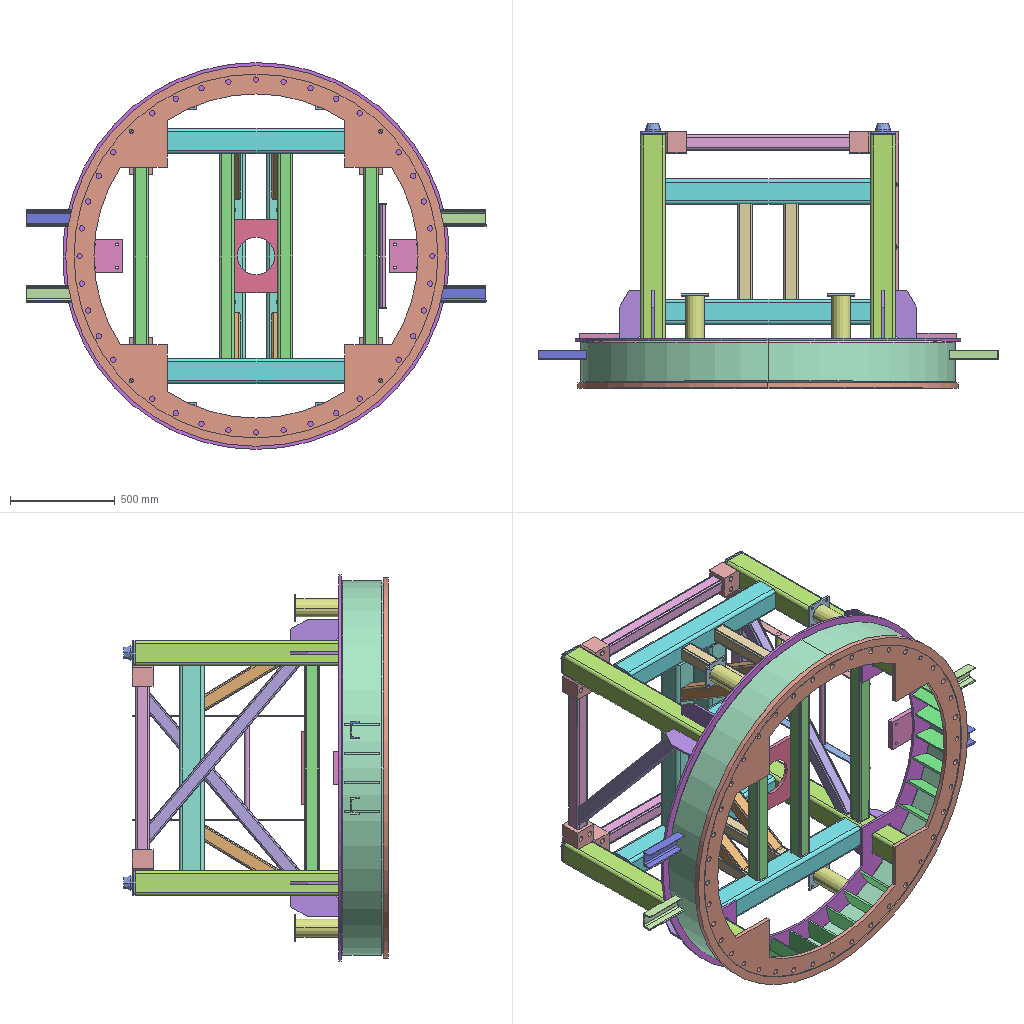Assembly | SolidWorks | 20 different items | 95 placed | box 2200 x 1265 x 1850 mm
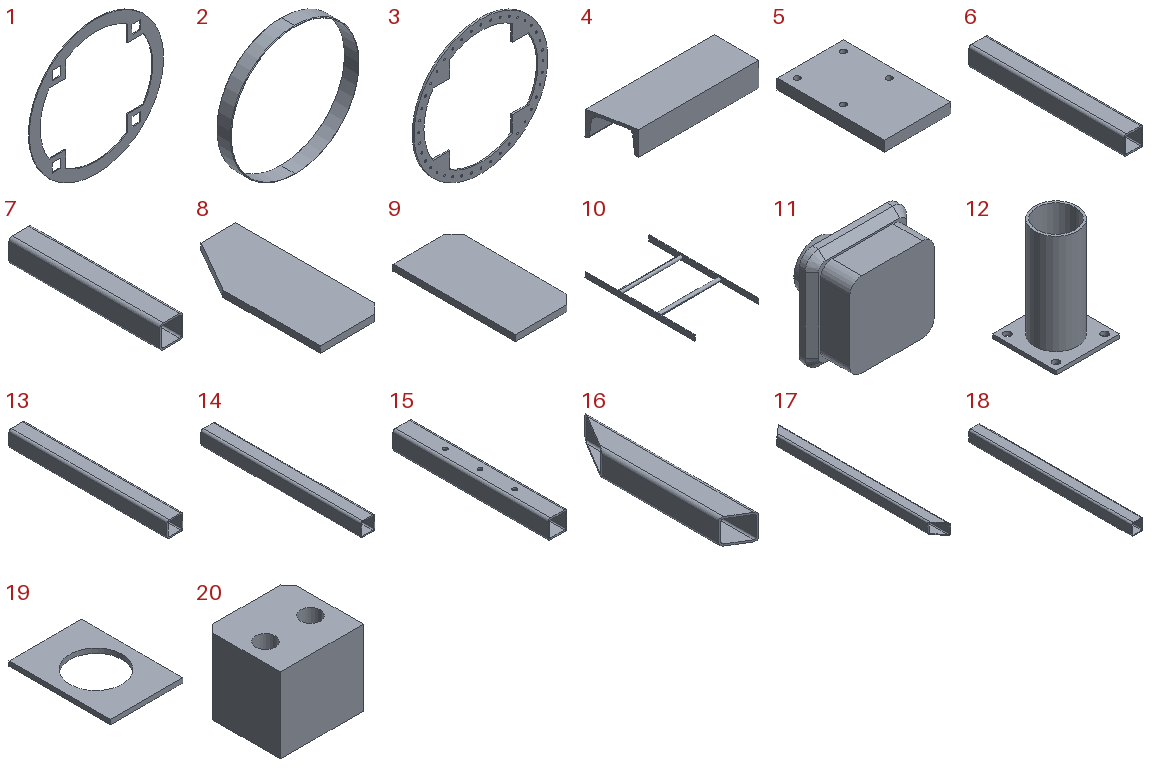Parts list (item | quantity | size | volume | features):
1 | x1 | 1850 x 12 x 1850 mm | 10257241 mm3 | features Extrusion 1
2 | x1 | 1790 x 200 x 1790 mm | 10805865 mm3 | features Chamfer 2, FlatPattern 1, SMBaseFlange 1, SheetMetal 1
3 | x1 | 1820 x 25 x 1820 mm | 17265104 mm3 | features HoleWzd 2, CirPattern 1, Extrusion 1, ICE 1
4 | x4 | 232.5 x 80 x 43 mm | 229319 mm3 | features ICE 2, WeldMemberFeat 1, WeldmentFeature 1
5 | x2 | 160 x 260 x 25 mm | 1024606 mm3 | features Extrusion 1, HoleWzd 1
6 | x4 | 120 x 980 x 120 mm | 4126927 mm3 | features WeldMemberFeat 1, WeldmentFeature 1
7 | x4 | 70 x 455 x 70 mm | 562207 mm3 | features WeldMemberFeat 1, WeldmentFeature 1
8 | x8 | 100 x 230 x 10 mm | 210475 mm3 | features Chamfer 1, Extrusion 1
9 | x32 | 100 x 200 x 10 mm | 197750 mm3 | features Chamfer 1, Extrusion 1, ICE 1
10 | x1 | 500 x 850 x 40 mm | 626926 mm3 | features WeldMemberFeat 2, WeldmentFeature 1
11 | x4 | 120 x 90 x 120 mm | 672208 mm3 | features Chamfer 2, ICE 2, Revolution 1
12 | x4 | 130 x 130 x 213 mm | 400765 mm3 | features Extrusion 1, WeldMemberFeat 1, WeldmentFeature 1
13 | x4 | 120 x 1185 x 120 mm | 4990213 mm3 | features WeldMemberFeat 1, WeldmentFeature 1
14 | x4 | 70 x 780 x 70 mm | 963783 mm3 | features WeldMemberFeat 1, WeldmentFeature 1
15 | x2 | 120 x 980 x 120 mm | 4095072 mm3 | features HoleWzd 1, WeldMemberFeat 1, WeldmentFeature 1
16 | x4 | 70 x 476 x 70 mm | 490129 mm3 | features ICE 1, WeldMemberFeat 1, WeldmentFeature 1
17 | x2 | 70 x 1116 x 70 mm | 1291200 mm3 | features ICE 1, WeldMemberFeat 1, WeldmentFeature 1
18 | x4 | 70 x 980 x 70 mm | 1210907 mm3 | features WeldMemberFeat 1, WeldmentFeature 1
19 | x1 | 250 x 350 x 16 mm | 992850 mm3 | features Extrusion 1
20 | x8 | 110 x 100 x 100 mm | 983814 mm3 | features Chamfer 1, Extrusion 1, HoleWzd 1
Mates (type | each side: item.copy, entity, surface, feature):
Coincident | 3.1 face plane Boss-Extrude 1 | assembly plane
Coincident | 3.1 plane | assembly plane | 2 times
Concentric | 2.1 face cylinder BaseBend1 | 3.1 face cylinder Boss-Extrude 1
Coincident | 2.1 face plane BaseBend1 | 3.1 face plane Boss-Extrude 1
Coincident | 2.1 plane | assembly plane
Concentric | 1.1 face cylinder Boss-Extrude 1 | 2.1 face cylinder BaseBend1
Coincident | 1.1 face plane Boss-Extrude 1 | 2.1 face plane BaseBend1
Coincident | 1.1 plane | assembly plane
Coincident | 1.1 face plane Boss-Extrude 1 | 12.1 face plane Round Tube 89X5(1)
Parallel | 12.1 face plane Boss-Extrude 1 | assembly plane
DistanceDim | 12.2 face cylinder Round Tube 89X5(1) | 12.3 face cylinder Round Tube 89X5(1)
DistanceDim | 12.2 face cylinder Round Tube 89X5(1) | 12.1 face cylinder Round Tube 89X5(1)
Width | 13.1 face plane Cold-Formed Square Hollow Section(gb t6728-2002) 120×120×10(1) | 13.1 face plane Cold-Formed Square Hollow Section(gb t6728-2002) 120×120×10(1) | 1.1 face plane Boss-Extrude 1 | 1.1 face plane Boss-Extrude 1 | 2 times
Coincident | 3.1 face plane Boss-Extrude 1 | 13.1 face plane Cold-Formed Square Hollow Section(gb t6728-2002) 120×120×10(1)
Width | 13.1 face plane Cold-Formed Square Hollow Section(gb t6728-2002) 120×120×10(1) | 13.1 face plane Cold-Formed Square Hollow Section(gb t6728-2002) 120×120×10(1) | 11.1 face plane Boss-Extrude 2 | 11.1 face plane Boss-Extrude 2
Width | 11.1 face plane Boss-Extrude 2 | 11.1 face plane Boss-Extrude 2 | 13.1 face plane Cold-Formed Square Hollow Section(gb t6728-2002) 120×120×10(1) | 13.1 face plane Cold-Formed Square Hollow Section(gb t6728-2002) 120×120×10(1)
Coincident | 13.1 face plane Cold-Formed Square Hollow Section(gb t6728-2002) 120×120×10(1) | 11.1 face plane Boss-Extrude 1
Width | 8.1 face plane Boss-Extrude 1 | 8.1 face plane Boss-Extrude 1 | 13.1 face plane Cold-Formed Square Hollow Section(gb t6728-2002) 120×120×10(1) | 13.1 face plane Cold-Formed Square Hollow Section(gb t6728-2002) 120×120×10(1)
Width | 8.2 face plane Boss-Extrude 1 | 8.2 face plane Boss-Extrude 1 | 13.1 face plane Cold-Formed Square Hollow Section(gb t6728-2002) 120×120×10(1) | 13.1 face plane Cold-Formed Square Hollow Section(gb t6728-2002) 120×120×10(1)
Coincident | 8.1 face plane Boss-Extrude 1 | 8.2 face plane Boss-Extrude 1
Coincident | 13.1 face plane Cold-Formed Square Hollow Section(gb t6728-2002) 120×120×10(1) | 8.2 face plane Boss-Extrude 1
Coincident | 13.1 face plane Cold-Formed Square Hollow Section(gb t6728-2002) 120×120×10(1) | 8.1 face plane Boss-Extrude 1
Coincident | 1.1 face plane Boss-Extrude 1 | 8.2 face plane Boss-Extrude 1
Coincident | 13.1 face plane Cold-Formed Square Hollow Section(gb t6728-2002) 120×120×10(1) | 20.1 face plane Boss-Extrude 1
Width | 20.1 face plane Boss-Extrude 1 | 20.1 face plane Boss-Extrude 1 | 13.1 face plane Cold-Formed Square Hollow Section(gb t6728-2002) 120×120×10(1) | 13.1 face plane Cold-Formed Square Hollow Section(gb t6728-2002) 120×120×10(1)
Coincident | 11.1 face plane Boss-Extrude 1 | 20.1 face plane Boss-Extrude 1
Coincident | 13.1 face plane Cold-Formed Square Hollow Section(gb t6728-2002) 120×120×10(1) | 20.2 face plane Boss-Extrude 1
Coincident | 20.1 face plane Boss-Extrude 1 | 20.2 face plane Boss-Extrude 1
Width | 20.2 face plane Boss-Extrude 1 | 20.2 face plane Boss-Extrude 1 | 13.1 face plane Cold-Formed Square Hollow Section(gb t6728-2002) 120×120×10(1) | 13.1 face plane Cold-Formed Square Hollow Section(gb t6728-2002) 120×120×10(1)
Width | 14.1 face plane Cold-Formed Square Hollow Section(gb t6728-2002) 70×70×5(1) | 14.1 face plane Cold-Formed Square Hollow Section(gb t6728-2002) 70×70×5(1) | 20.1 face plane Boss-Extrude 1 | 20.1 face plane Boss-Extrude 1 | 2 times
Coincident | 14.1 face plane Cold-Formed Square Hollow Section(gb t6728-2002) 70×70×5(1) | 20.1 face plane Boss-Extrude 1
Coincident | 13.1 face plane Cold-Formed Square Hollow Section(gb t6728-2002) 120×120×10(1) | 6.1 face plane Cold-Formed Square Hollow Section(gb t6728-2002) 120×120×10(1) | 2 times
DistanceDim | 6.2 face plane Cold-Formed Square Hollow Section(gb t6728-2002) 120×120×10(1) | 1.1 face plane Boss-Extrude 1
Coincident | 13.1 face plane Cold-Formed Square Hollow Section(gb t6728-2002) 120×120×10(1) | 6.2 face plane Cold-Formed Square Hollow Section(gb t6728-2002) 120×120×10(1)
Coincident | 6.1 face plane Cold-Formed Square Hollow Section(gb t6728-2002) 120×120×10(1) | 6.2 face plane Cold-Formed Square Hollow Section(gb t6728-2002) 120×120×10(1)
DistanceDim | 6.1 face plane Cold-Formed Square Hollow Section(gb t6728-2002) 120×120×10(1) | 6.2 face plane Cold-Formed Square Hollow Section(gb t6728-2002) 120×120×10(1)
DistanceDim | 6.3 face plane Cold-Formed Square Hollow Section(gb t6728-2002) 120×120×10(1) | 6.4 face plane Cold-Formed Square Hollow Section(gb t6728-2002) 120×120×10(1)
Coincident | 6.4 face plane Cold-Formed Square Hollow Section(gb t6728-2002) 120×120×10(1) | 6.3 face plane Cold-Formed Square Hollow Section(gb t6728-2002) 120×120×10(1) | 2 times
Coincident | 13.2 face plane Cold-Formed Square Hollow Section(gb t6728-2002) 120×120×10(1) | 6.3 face plane Cold-Formed Square Hollow Section(gb t6728-2002) 120×120×10(1) | 2 times
Coincident | 6.1 face plane Cold-Formed Square Hollow Section(gb t6728-2002) 120×120×10(1) | 6.3 face plane Cold-Formed Square Hollow Section(gb t6728-2002) 120×120×10(1)
Width | 7.1 face plane Cold-Formed Square Hollow Section(gb t6728-2002) 70×70×5(1) | 7.1 face plane Cold-Formed Square Hollow Section(gb t6728-2002) 70×70×5(1) | 6.2 face plane Cold-Formed Square Hollow Section(gb t6728-2002) 120×120×10(1) | 6.2 face plane Cold-Formed Square Hollow Section(gb t6728-2002) 120×120×10(1)
Coincident | 7.1 face plane Cold-Formed Square Hollow Section(gb t6728-2002) 70×70×5(1) | 7.2 face plane Cold-Formed Square Hollow Section(gb t6728-2002) 70×70×5(1) | 2 times
Coincident | 15.1 face plane Cold-Formed Square Hollow Section(gb t6728-2002) 120×120×10(1) | 15.2 face plane Cold-Formed Square Hollow Section(gb t6728-2002) 120×120×10(1) | 2 times
Coincident | 6.1 face plane Cold-Formed Square Hollow Section(gb t6728-2002) 120×120×10(1) | 15.1 face plane Cold-Formed Square Hollow Section(gb t6728-2002) 120×120×10(1) | 2 times
DistanceDim | 15.2 face plane Cold-Formed Square Hollow Section(gb t6728-2002) 120×120×10(1) | 15.1 face plane Cold-Formed Square Hollow Section(gb t6728-2002) 120×120×10(1)
Symmetric | 15.1 face plane Cold-Formed Square Hollow Section(gb t6728-2002) 120×120×10(1) | 15.2 face plane Cold-Formed Square Hollow Section(gb t6728-2002) 120×120×10(1) | assembly plane
Coincident | 1.1 face plane Boss-Extrude 1 | 9.1 face plane Boss-Extrude 1
Coincident | 9.1 plane | assembly select_type:10
Coincident | 2.1 face cylinder BaseBend1 | 9.1 edge
Coincident | 13.1 face plane Cold-Formed Square Hollow Section(gb t6728-2002) 120×120×10(1) | 17.1 face plane Cut-Extrude 1
Coincident | 14.2 face plane Cold-Formed Square Hollow Section(gb t6728-2002) 70×70×5(1) | 17.1 face plane Cut-Extrude 1
Coincident | 14.2 face plane Cold-Formed Square Hollow Section(gb t6728-2002) 70×70×5(1) | 17.1 face plane Cold-Formed Square Hollow Section(gb t6728-2002) 70×70×5(1)
Width | 7.1 face plane Cold-Formed Square Hollow Section(gb t6728-2002) 70×70×5(1) | 7.1 face plane Cold-Formed Square Hollow Section(gb t6728-2002) 70×70×5(1) | 15.1 face plane Cold-Formed Square Hollow Section(gb t6728-2002) 120×120×10(1) | 15.1 face plane Cold-Formed Square Hollow Section(gb t6728-2002) 120×120×10(1)
Width | 7.2 face plane Cold-Formed Square Hollow Section(gb t6728-2002) 70×70×5(1) | 7.2 face plane Cold-Formed Square Hollow Section(gb t6728-2002) 70×70×5(1) | 15.2 face plane Cold-Formed Square Hollow Section(gb t6728-2002) 120×120×10(1) | 15.2 face plane Cold-Formed Square Hollow Section(gb t6728-2002) 120×120×10(1)
Coincident | 6.1 face plane Cold-Formed Square Hollow Section(gb t6728-2002) 120×120×10(1) | 7.2 face plane Cold-Formed Square Hollow Section(gb t6728-2002) 70×70×5(1)
Coincident | 7.1 face plane Cold-Formed Square Hollow Section(gb t6728-2002) 70×70×5(1) | 16.1 face plane Cut-Extrude 1
Coincident | 15.1 face plane Cold-Formed Square Hollow Section(gb t6728-2002) 120×120×10(1) | 16.1 face plane Cut-Extrude 1
Coincident | 7.1 face plane Cold-Formed Square Hollow Section(gb t6728-2002) 70×70×5(1) | 16.1 face plane Cold-Formed Square Hollow Section(gb t6728-2002) 70×70×5(1)
Coincident | 16.1 face plane Cut-Extrude 1 | 16.2 face plane Cut-Extrude 1 | 2 times
Coincident | 7.2 face plane Cold-Formed Square Hollow Section(gb t6728-2002) 70×70×5(1) | 16.2 face plane Cold-Formed Square Hollow Section(gb t6728-2002) 70×70×5(1)
Coincident | 18.1 face plane Cold-Formed Square Hollow Section(gb t6728-2002) 70×70×5(1) | 13.2 face plane Cold-Formed Square Hollow Section(gb t6728-2002) 120×120×10(1)
Width | 18.1 face plane Cold-Formed Square Hollow Section(gb t6728-2002) 70×70×5(1) | 18.1 face plane Cold-Formed Square Hollow Section(gb t6728-2002) 70×70×5(1) | 13.2 face plane Cold-Formed Square Hollow Section(gb t6728-2002) 120×120×10(1) | 13.2 face plane Cold-Formed Square Hollow Section(gb t6728-2002) 120×120×10(1)
DistanceDim | 1.1 face plane Boss-Extrude 1 | 18.1 face plane Cold-Formed Square Hollow Section(gb t6728-2002) 70×70×5(1)
Coincident | 4.1 face plane Hot-Rolled Channel Steel(gb t707-1988) 8-XXXXXXXXXXXXXXX528V9(1) | 4.2 face plane Hot-Rolled Channel Steel(gb t707-1988) 8-XXXXXXXXXXXXXXX528V9(1) | 2 times
DistanceDim | 4.1 face plane Hot-Rolled Channel Steel(gb t707-1988) 8-XXXXXXXXXXXXXXX528V9(1) | 4.2 face plane Hot-Rolled Channel Steel(gb t707-1988) 8-XXXXXXXXXXXXXXX528V9(1)
Symmetric | 4.1 face plane Hot-Rolled Channel Steel(gb t707-1988) 8-XXXXXXXXXXXXXXX528V9(1) | 4.2 face plane Hot-Rolled Channel Steel(gb t707-1988) 8-XXXXXXXXXXXXXXX528V9(1) | assembly plane
DistanceDim | 4.1 face plane Hot-Rolled Channel Steel(gb t707-1988) 8-XXXXXXXXXXXXXXX528V9(1) | 3.1 face plane Boss-Extrude 1
Coincident | 2.1 face cylinder BaseBend1 | 4.1 edge
Coincident | 1.1 face plane Boss-Extrude 1 | 5.1 face plane Boss-Extrude 1
Coincident | 5.1 plane | assembly plane
DistanceDim | 5.1 face plane Boss-Extrude 1 | 5.2 face plane Boss-Extrude 1
Coincident | 14.3 face plane Cold-Formed Square Hollow Section(gb t6728-2002) 70×70×5(1) | 17.2 face plane Cut-Extrude 1
Coincident | 13.3 face plane Cold-Formed Square Hollow Section(gb t6728-2002) 120×120×10(1) | 17.2 face plane Cut-Extrude 1
Width | 17.2 face plane Cold-Formed Square Hollow Section(gb t6728-2002) 70×70×5(1) | 17.2 face plane Cold-Formed Square Hollow Section(gb t6728-2002) 70×70×5(1) | 13.3 face plane Cold-Formed Square Hollow Section(gb t6728-2002) 120×120×10(1) | 13.3 face plane Cold-Formed Square Hollow Section(gb t6728-2002) 120×120×10(1)
Coincident | 18.1 face plane Cold-Formed Square Hollow Section(gb t6728-2002) 70×70×5(1) | 18.2 face plane Cold-Formed Square Hollow Section(gb t6728-2002) 70×70×5(1)
Coincident | 6.2 face plane Cold-Formed Square Hollow Section(gb t6728-2002) 120×120×10(1) | 18.2 face plane Cold-Formed Square Hollow Section(gb t6728-2002) 70×70×5(1)
Coincident | 19.1 face plane Boss-Extrude 1 | 18.2 face plane Cold-Formed Square Hollow Section(gb t6728-2002) 70×70×5(1)
Coincident | 19.1 plane | assembly plane | 2 times
DistanceDim | 18.2 face plane Cold-Formed Square Hollow Section(gb t6728-2002) 70×70×5(1) | 18.1 face plane Cold-Formed Square Hollow Section(gb t6728-2002) 70×70×5(1)
Coincident | 14.3 face plane Cold-Formed Square Hollow Section(gb t6728-2002) 70×70×5(1) | 10.1 face plane Gb/t 704—1988Hot-Rolled Flat Steel 40×6(1)
Coincident | 10.1 plane | assembly plane
DistanceDim | 10.1 face plane Gb/t 704—1988Hot-Rolled Flat Steel 40×6(1) | 14.3 face plane Cold-Formed Square Hollow Section(gb t6728-2002) 70×70×5(1)